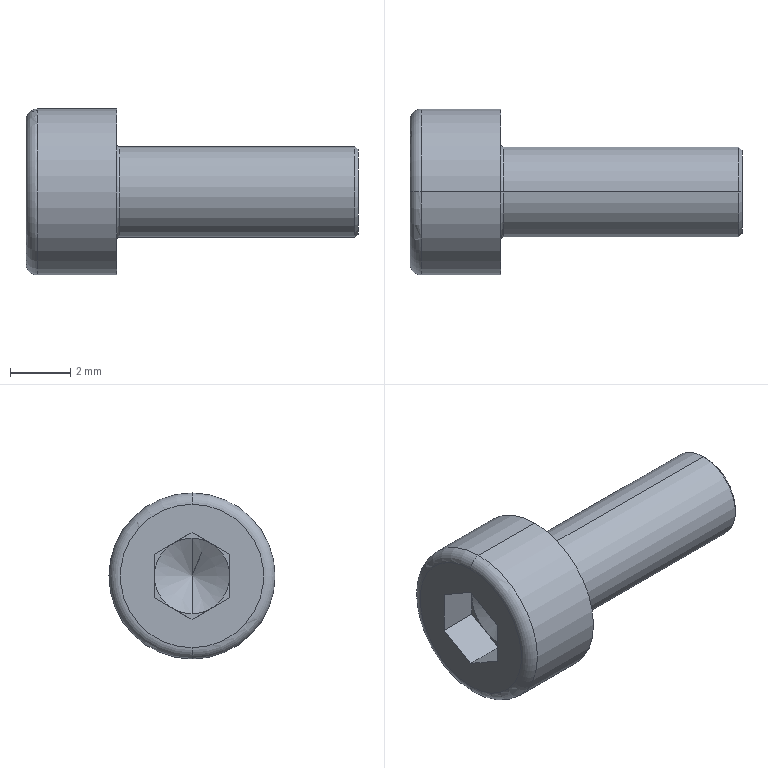Part | STEP file | 1 solid | 27 faces | box 11 x 5.5 x 5.5 mm | volume 119.075 mm3 | plane 15 | torus 4 | cone 4 | cylinder 4 | commonest cylinder face diameters 3 x2 5.5 x2